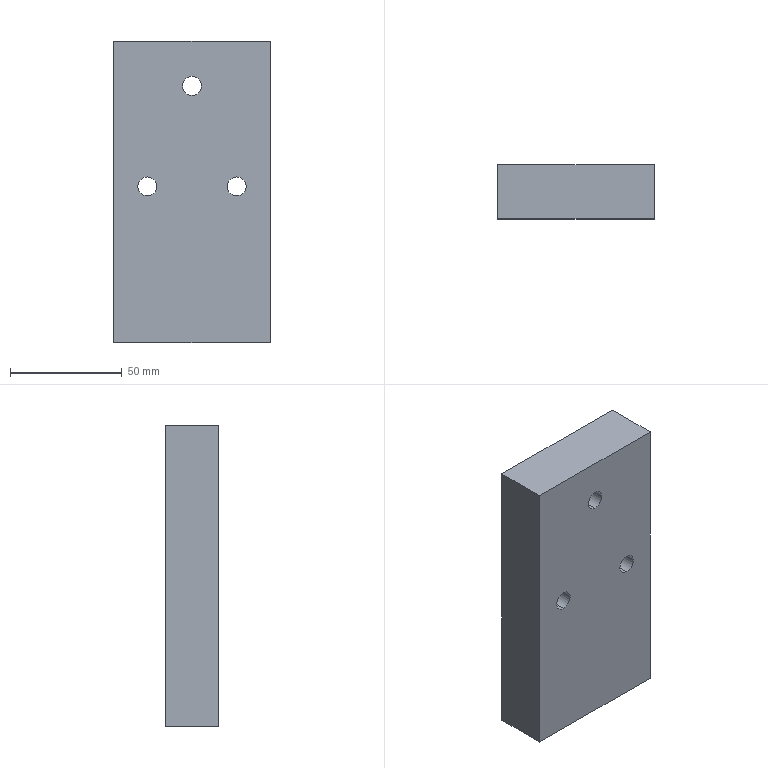Part | SolidWorks | features Extrusion 1, HoleWzd 1 | 1 solid | 12 faces | box 70 x 24 x 135 mm | volume 222714 mm3 | cylinder 6 | plane 6 | commonest cylinder face diameters 8.5 x6
STEP:
#1=CARTESIAN_POINT('',(-20.,0.,-1.75));
#2=VERTEX_POINT('',#1);
#3=CARTESIAN_POINT('',(-20.,0.,6.75));
#4=VERTEX_POINT('',#3);
#5=CARTESIAN_POINT('',(-20.,0.,2.5));
#6=DIRECTION('',(0.,1.,0.));
#7=DIRECTION('',(0.,0.,1.));
#8=AXIS2_PLACEMENT_3D('',#5,#6,#7);
#9=CIRCLE('',#8,4.25);
#10=EDGE_CURVE('',#2,#4,#9,.T.);
#11=ORIENTED_EDGE('',*,*,#10,.F.);
#12=CARTESIAN_POINT('',(-20.,24.,-1.75));
#13=VERTEX_POINT('',#12);
#14=CARTESIAN_POINT('',(-20.,24.,-1.75));
#15=DIRECTION('',(0.,1.,0.));
#16=VECTOR('',#15,1000.);
#17=LINE('',#14,#16);
#18=EDGE_CURVE('',#2,#13,#17,.T.);
#19=ORIENTED_EDGE('',*,*,#18,.T.);
#20=CARTESIAN_POINT('',(-20.,24.,6.75));
#21=VERTEX_POINT('',#20);
#22=CARTESIAN_POINT('',(-20.,24.,2.5));
#23=DIRECTION('',(0.,1.,0.));
#24=DIRECTION('',(0.,0.,1.));
#25=AXIS2_PLACEMENT_3D('',#22,#23,#24);
#26=CIRCLE('',#25,4.25);
#27=EDGE_CURVE('',#13,#21,#26,.T.);
#28=ORIENTED_EDGE('',*,*,#27,.T.);
#29=CARTESIAN_POINT('',(-20.,24.,6.75));
#30=DIRECTION('',(0.,1.,0.));
#31=VECTOR('',#30,1000.);
#32=LINE('',#29,#31);
#33=EDGE_CURVE('',#4,#21,#32,.T.);
#34=ORIENTED_EDGE('',*,*,#33,.F.);
#35=EDGE_LOOP('',(#11,#19,#28,#34));
#36=FACE_OUTER_BOUND('',#35,.T.);
#37=CARTESIAN_POINT('',(-20.,24.,2.5));
#38=DIRECTION('',(0.,1.,0.));
#39=DIRECTION('',(0.,0.,1.));
#40=AXIS2_PLACEMENT_3D('',#37,#38,#39);
#41=CYLINDRICAL_SURFACE('',#40,4.25);
#42=ADVANCED_FACE('',(#36),#41,.F.);
#43=CARTESIAN_POINT('',(20.,0.,-1.75));
#44=VERTEX_POINT('',#43);
#45=CARTESIAN_POINT('',(20.,0.,6.75));
#46=VERTEX_POINT('',#45);
#47=CARTESIAN_POINT('',(20.,0.,2.5));
#48=DIRECTION('',(0.,1.,0.));
#49=DIRECTION('',(0.,0.,1.));
#50=AXIS2_PLACEMENT_3D('',#47,#48,#49);
#51=CIRCLE('',#50,4.25);
#52=EDGE_CURVE('',#44,#46,#51,.T.);
#53=ORIENTED_EDGE('',*,*,#52,.F.);
#54=CARTESIAN_POINT('',(20.,24.,-1.75));
#55=VERTEX_POINT('',#54);
#56=CARTESIAN_POINT('',(20.,24.,-1.75));
#57=DIRECTION('',(0.,1.,0.));
#58=VECTOR('',#57,1000.);
#59=LINE('',#56,#58);
#60=EDGE_CURVE('',#44,#55,#59,.T.);
#61=ORIENTED_EDGE('',*,*,#60,.T.);
#62=CARTESIAN_POINT('',(20.,24.,6.75));
#63=VERTEX_POINT('',#62);
#64=CARTESIAN_POINT('',(20.,24.,2.5));
#65=DIRECTION('',(0.,1.,0.));
#66=DIRECTION('',(0.,0.,1.));
#67=AXIS2_PLACEMENT_3D('',#64,#65,#66);
#68=CIRCLE('',#67,4.25);
#69=EDGE_CURVE('',#55,#63,#68,.T.);
#70=ORIENTED_EDGE('',*,*,#69,.T.);
#71=CARTESIAN_POINT('',(20.,24.,6.75));
#72=DIRECTION('',(0.,1.,0.));
#73=VECTOR('',#72,1000.);
#74=LINE('',#71,#73);
#75=EDGE_CURVE('',#46,#63,#74,.T.);
#76=ORIENTED_EDGE('',*,*,#75,.F.);
#77=EDGE_LOOP('',(#53,#61,#70,#76));
#78=FACE_OUTER_BOUND('',#77,.T.);
#79=CARTESIAN_POINT('',(20.,24.,2.5));
#80=DIRECTION('',(0.,1.,0.));
#81=DIRECTION('',(0.,0.,1.));
#82=AXIS2_PLACEMENT_3D('',#79,#80,#81);
#83=CYLINDRICAL_SURFACE('',#82,4.25);
#84=ADVANCED_FACE('',(#78),#83,.F.);
#85=CARTESIAN_POINT('',(0.,0.,43.25));
#86=VERTEX_POINT('',#85);
#87=CARTESIAN_POINT('',(0.,0.,51.75));
#88=VERTEX_POINT('',#87);
#89=CARTESIAN_POINT('',(0.,0.,47.5));
#90=DIRECTION('',(0.,1.,0.));
#91=DIRECTION('',(0.,0.,1.));
#92=AXIS2_PLACEMENT_3D('',#89,#90,#91);
#93=CIRCLE('',#92,4.25);
#94=EDGE_CURVE('',#86,#88,#93,.T.);
#95=ORIENTED_EDGE('',*,*,#94,.F.);
#96=CARTESIAN_POINT('',(0.,24.,43.25));
#97=VERTEX_POINT('',#96);
#98=CARTESIAN_POINT('',(0.,24.,43.25));
#99=DIRECTION('',(0.,1.,0.));
#100=VECTOR('',#99,1000.);
#101=LINE('',#98,#100);
#102=EDGE_CURVE('',#86,#97,#101,.T.);
#103=ORIENTED_EDGE('',*,*,#102,.T.);
#104=CARTESIAN_POINT('',(0.,24.,51.75));
#105=VERTEX_POINT('',#104);
#106=CARTESIAN_POINT('',(0.,24.,47.5));
#107=DIRECTION('',(0.,1.,0.));
#108=DIRECTION('',(0.,0.,1.));
#109=AXIS2_PLACEMENT_3D('',#106,#107,#108);
#110=CIRCLE('',#109,4.25);
#111=EDGE_CURVE('',#97,#105,#110,.T.);
#112=ORIENTED_EDGE('',*,*,#111,.T.);
#113=CARTESIAN_POINT('',(0.,24.,51.75));
#114=DIRECTION('',(0.,1.,0.));
#115=VECTOR('',#114,1000.);
#116=LINE('',#113,#115);
#117=EDGE_CURVE('',#88,#105,#116,.T.);
#118=ORIENTED_EDGE('',*,*,#117,.F.);
#119=EDGE_LOOP('',(#95,#103,#112,#118));
#120=FACE_OUTER_BOUND('',#119,.T.);
#121=CARTESIAN_POINT('',(0.,24.,47.5));
#122=DIRECTION('',(0.,1.,0.));
#123=DIRECTION('',(0.,0.,1.));
#124=AXIS2_PLACEMENT_3D('',#121,#122,#123);
#125=CYLINDRICAL_SURFACE('',#124,4.25);
#126=ADVANCED_FACE('',(#120),#125,.F.);
#127=CARTESIAN_POINT('',(35.,0.,67.5));
#128=VERTEX_POINT('',#127);
#129=CARTESIAN_POINT('',(35.,0.,-67.5));
#130=VERTEX_POINT('',#129);
#131=CARTESIAN_POINT('',(35.,0.,67.5));
#132=DIRECTION('',(0.,0.,-1.));
#133=VECTOR('',#132,1000.);
#134=LINE('',#131,#133);
#135=EDGE_CURVE('',#128,#130,#134,.T.);
#136=ORIENTED_EDGE('',*,*,#135,.T.);
#137=CARTESIAN_POINT('',(35.,24.,-67.5));
#138=VERTEX_POINT('',#137);
#139=CARTESIAN_POINT('',(35.,24.,-67.5));
#140=DIRECTION('',(0.,-1.,0.));
#141=VECTOR('',#140,1000.);
#142=LINE('',#139,#141);
#143=EDGE_CURVE('',#138,#130,#142,.T.);
#144=ORIENTED_EDGE('',*,*,#143,.F.);
#145=CARTESIAN_POINT('',(35.,24.,67.5));
#146=VERTEX_POINT('',#145);
#147=CARTESIAN_POINT('',(35.,24.,67.5));
#148=DIRECTION('',(0.,0.,-1.));
#149=VECTOR('',#148,1000.);
#150=LINE('',#147,#149);
#151=EDGE_CURVE('',#146,#138,#150,.T.);
#152=ORIENTED_EDGE('',*,*,#151,.F.);
#153=CARTESIAN_POINT('',(35.,24.,67.5));
#154=DIRECTION('',(0.,-1.,0.));
#155=VECTOR('',#154,1000.);
#156=LINE('',#153,#155);
#157=EDGE_CURVE('',#146,#128,#156,.T.);
#158=ORIENTED_EDGE('',*,*,#157,.T.);
#159=EDGE_LOOP('',(#136,#144,#152,#158));
#160=FACE_OUTER_BOUND('',#159,.T.);
#161=CARTESIAN_POINT('',(35.,24.,67.5));
#162=DIRECTION('',(-1.,0.,0.));
#163=DIRECTION('',(0.,0.,1.));
#164=AXIS2_PLACEMENT_3D('',#161,#162,#163);
#165=PLANE('',#164);
#166=ADVANCED_FACE('',(#160),#165,.F.);
#167=CARTESIAN_POINT('',(-35.,0.,-67.5));
#168=VERTEX_POINT('',#167);
#169=CARTESIAN_POINT('',(-35.,0.,-67.5));
#170=DIRECTION('',(-1.,0.,0.));
#171=VECTOR('',#170,1000.);
#172=LINE('',#169,#171);
#173=EDGE_CURVE('',#130,#168,#172,.T.);
#174=ORIENTED_EDGE('',*,*,#173,.T.);
#175=CARTESIAN_POINT('',(-35.,24.,-67.5));
#176=VERTEX_POINT('',#175);
#177=CARTESIAN_POINT('',(-35.,24.,-67.5));
#178=DIRECTION('',(0.,-1.,0.));
#179=VECTOR('',#178,1000.);
#180=LINE('',#177,#179);
#181=EDGE_CURVE('',#176,#168,#180,.T.);
#182=ORIENTED_EDGE('',*,*,#181,.F.);
#183=CARTESIAN_POINT('',(-35.,24.,-67.5));
#184=DIRECTION('',(-1.,0.,0.));
#185=VECTOR('',#184,1000.);
#186=LINE('',#183,#185);
#187=EDGE_CURVE('',#138,#176,#186,.T.);
#188=ORIENTED_EDGE('',*,*,#187,.F.);
#189=ORIENTED_EDGE('',*,*,#143,.T.);
#190=EDGE_LOOP('',(#174,#182,#188,#189));
#191=FACE_OUTER_BOUND('',#190,.T.);
#192=CARTESIAN_POINT('',(-35.,24.,-67.5));
#193=DIRECTION('',(0.,0.,1.));
#194=DIRECTION('',(1.,0.,0.));
#195=AXIS2_PLACEMENT_3D('',#192,#193,#194);
#196=PLANE('',#195);
#197=ADVANCED_FACE('',(#191),#196,.F.);
#198=CARTESIAN_POINT('',(-35.,0.,67.5));
#199=VERTEX_POINT('',#198);
#200=CARTESIAN_POINT('',(-35.,0.,67.5));
#201=DIRECTION('',(0.,0.,1.));
#202=VECTOR('',#201,1000.);
#203=LINE('',#200,#202);
#204=EDGE_CURVE('',#168,#199,#203,.T.);
#205=ORIENTED_EDGE('',*,*,#204,.T.);
#206=CARTESIAN_POINT('',(-35.,24.,67.5));
#207=VERTEX_POINT('',#206);
#208=CARTESIAN_POINT('',(-35.,24.,67.5));
#209=DIRECTION('',(0.,-1.,0.));
#210=VECTOR('',#209,1000.);
#211=LINE('',#208,#210);
#212=EDGE_CURVE('',#207,#199,#211,.T.);
#213=ORIENTED_EDGE('',*,*,#212,.F.);
#214=CARTESIAN_POINT('',(-35.,24.,67.5));
#215=DIRECTION('',(0.,0.,1.));
#216=VECTOR('',#215,1000.);
#217=LINE('',#214,#216);
#218=EDGE_CURVE('',#176,#207,#217,.T.);
#219=ORIENTED_EDGE('',*,*,#218,.F.);
#220=ORIENTED_EDGE('',*,*,#181,.T.);
#221=EDGE_LOOP('',(#205,#213,#219,#220));
#222=FACE_OUTER_BOUND('',#221,.T.);
#223=CARTESIAN_POINT('',(-35.,24.,67.5));
#224=DIRECTION('',(1.,0.,0.));
#225=DIRECTION('',(0.,0.,-1.));
#226=AXIS2_PLACEMENT_3D('',#223,#224,#225);
#227=PLANE('',#226);
#228=ADVANCED_FACE('',(#222),#227,.F.);
#229=CARTESIAN_POINT('',(-35.,0.,67.5));
#230=DIRECTION('',(1.,0.,0.));
#231=VECTOR('',#230,1000.);
#232=LINE('',#229,#231);
#233=EDGE_CURVE('',#199,#128,#232,.T.);
#234=ORIENTED_EDGE('',*,*,#233,.T.);
#235=ORIENTED_EDGE('',*,*,#157,.F.);
#236=CARTESIAN_POINT('',(-35.,24.,67.5));
#237=DIRECTION('',(1.,0.,0.));
#238=VECTOR('',#237,1000.);
#239=LINE('',#236,#238);
#240=EDGE_CURVE('',#207,#146,#239,.T.);
#241=ORIENTED_EDGE('',*,*,#240,.F.);
#242=ORIENTED_EDGE('',*,*,#212,.T.);
#243=EDGE_LOOP('',(#234,#235,#241,#242));
#244=FACE_OUTER_BOUND('',#243,.T.);
#245=CARTESIAN_POINT('',(-35.,24.,67.5));
#246=DIRECTION('',(0.,0.,-1.));
#247=DIRECTION('',(-1.,0.,0.));
#248=AXIS2_PLACEMENT_3D('',#245,#246,#247);
#249=PLANE('',#248);
#250=ADVANCED_FACE('',(#244),#249,.F.);
#251=CARTESIAN_POINT('',(-20.,24.,2.5));
#252=DIRECTION('',(0.,1.,0.));
#253=DIRECTION('',(0.,0.,1.));
#254=AXIS2_PLACEMENT_3D('',#251,#252,#253);
#255=CIRCLE('',#254,4.25);
#256=EDGE_CURVE('',#21,#13,#255,.T.);
#257=ORIENTED_EDGE('',*,*,#256,.F.);
#258=ORIENTED_EDGE('',*,*,#27,.F.);
#259=EDGE_LOOP('',(#257,#258));
#260=FACE_BOUND('',#259,.T.);
#261=CARTESIAN_POINT('',(20.,24.,2.5));
#262=DIRECTION('',(0.,1.,0.));
#263=DIRECTION('',(0.,0.,1.));
#264=AXIS2_PLACEMENT_3D('',#261,#262,#263);
#265=CIRCLE('',#264,4.25);
#266=EDGE_CURVE('',#63,#55,#265,.T.);
#267=ORIENTED_EDGE('',*,*,#266,.F.);
#268=ORIENTED_EDGE('',*,*,#69,.F.);
#269=EDGE_LOOP('',(#267,#268));
#270=FACE_BOUND('',#269,.T.);
#271=CARTESIAN_POINT('',(0.,24.,47.5));
#272=DIRECTION('',(0.,1.,0.));
#273=DIRECTION('',(0.,0.,1.));
#274=AXIS2_PLACEMENT_3D('',#271,#272,#273);
#275=CIRCLE('',#274,4.25);
#276=EDGE_CURVE('',#105,#97,#275,.T.);
#277=ORIENTED_EDGE('',*,*,#276,.F.);
#278=ORIENTED_EDGE('',*,*,#111,.F.);
#279=EDGE_LOOP('',(#277,#278));
#280=FACE_BOUND('',#279,.T.);
#281=ORIENTED_EDGE('',*,*,#151,.T.);
#282=ORIENTED_EDGE('',*,*,#187,.T.);
#283=ORIENTED_EDGE('',*,*,#218,.T.);
#284=ORIENTED_EDGE('',*,*,#240,.T.);
#285=EDGE_LOOP('',(#281,#282,#283,#284));
#286=FACE_OUTER_BOUND('',#285,.T.);
#287=CARTESIAN_POINT('',(0.,24.,0.));
#288=DIRECTION('',(0.,-1.,0.));
#289=DIRECTION('',(0.,0.,-1.));
#290=AXIS2_PLACEMENT_3D('',#287,#288,#289);
#291=PLANE('',#290);
#292=ADVANCED_FACE('',(#260,#270,#280,#286),#291,.F.);
#293=CARTESIAN_POINT('',(-20.,0.,2.5));
#294=DIRECTION('',(0.,1.,0.));
#295=DIRECTION('',(0.,0.,1.));
#296=AXIS2_PLACEMENT_3D('',#293,#294,#295);
#297=CIRCLE('',#296,4.25);
#298=EDGE_CURVE('',#4,#2,#297,.T.);
#299=ORIENTED_EDGE('',*,*,#298,.T.);
#300=ORIENTED_EDGE('',*,*,#10,.T.);
#301=EDGE_LOOP('',(#299,#300));
#302=FACE_BOUND('',#301,.T.);
#303=CARTESIAN_POINT('',(20.,0.,2.5));
#304=DIRECTION('',(0.,1.,0.));
#305=DIRECTION('',(0.,0.,1.));
#306=AXIS2_PLACEMENT_3D('',#303,#304,#305);
#307=CIRCLE('',#306,4.25);
#308=EDGE_CURVE('',#46,#44,#307,.T.);
#309=ORIENTED_EDGE('',*,*,#308,.T.);
#310=ORIENTED_EDGE('',*,*,#52,.T.);
#311=EDGE_LOOP('',(#309,#310));
#312=FACE_BOUND('',#311,.T.);
#313=CARTESIAN_POINT('',(0.,0.,47.5));
#314=DIRECTION('',(0.,1.,0.));
#315=DIRECTION('',(0.,0.,1.));
#316=AXIS2_PLACEMENT_3D('',#313,#314,#315);
#317=CIRCLE('',#316,4.25);
#318=EDGE_CURVE('',#88,#86,#317,.T.);
#319=ORIENTED_EDGE('',*,*,#318,.T.);
#320=ORIENTED_EDGE('',*,*,#94,.T.);
#321=EDGE_LOOP('',(#319,#320));
#322=FACE_BOUND('',#321,.T.);
#323=ORIENTED_EDGE('',*,*,#135,.F.);
#324=ORIENTED_EDGE('',*,*,#233,.F.);
#325=ORIENTED_EDGE('',*,*,#204,.F.);
#326=ORIENTED_EDGE('',*,*,#173,.F.);
#327=EDGE_LOOP('',(#323,#324,#325,#326));
#328=FACE_OUTER_BOUND('',#327,.T.);
#329=CARTESIAN_POINT('',(0.,0.,0.));
#330=DIRECTION('',(0.,-1.,0.));
#331=DIRECTION('',(0.,0.,-1.));
#332=AXIS2_PLACEMENT_3D('',#329,#330,#331);
#333=PLANE('',#332);
#334=ADVANCED_FACE('',(#302,#312,#322,#328),#333,.T.);
#335=ORIENTED_EDGE('',*,*,#102,.F.);
#336=ORIENTED_EDGE('',*,*,#318,.F.);
#337=ORIENTED_EDGE('',*,*,#117,.T.);
#338=ORIENTED_EDGE('',*,*,#276,.T.);
#339=EDGE_LOOP('',(#335,#336,#337,#338));
#340=FACE_OUTER_BOUND('',#339,.T.);
#341=CARTESIAN_POINT('',(0.,24.,47.5));
#342=DIRECTION('',(0.,1.,0.));
#343=DIRECTION('',(0.,0.,1.));
#344=AXIS2_PLACEMENT_3D('',#341,#342,#343);
#345=CYLINDRICAL_SURFACE('',#344,4.25);
#346=ADVANCED_FACE('',(#340),#345,.F.);
#347=ORIENTED_EDGE('',*,*,#60,.F.);
#348=ORIENTED_EDGE('',*,*,#308,.F.);
#349=ORIENTED_EDGE('',*,*,#75,.T.);
#350=ORIENTED_EDGE('',*,*,#266,.T.);
#351=EDGE_LOOP('',(#347,#348,#349,#350));
#352=FACE_OUTER_BOUND('',#351,.T.);
#353=CARTESIAN_POINT('',(20.,24.,2.5));
#354=DIRECTION('',(0.,1.,0.));
#355=DIRECTION('',(0.,0.,1.));
#356=AXIS2_PLACEMENT_3D('',#353,#354,#355);
#357=CYLINDRICAL_SURFACE('',#356,4.25);
#358=ADVANCED_FACE('',(#352),#357,.F.);
#359=ORIENTED_EDGE('',*,*,#18,.F.);
#360=ORIENTED_EDGE('',*,*,#298,.F.);
#361=ORIENTED_EDGE('',*,*,#33,.T.);
#362=ORIENTED_EDGE('',*,*,#256,.T.);
#363=EDGE_LOOP('',(#359,#360,#361,#362));
#364=FACE_OUTER_BOUND('',#363,.T.);
#365=CARTESIAN_POINT('',(-20.,24.,2.5));
#366=DIRECTION('',(0.,1.,0.));
#367=DIRECTION('',(0.,0.,1.));
#368=AXIS2_PLACEMENT_3D('',#365,#366,#367);
#369=CYLINDRICAL_SURFACE('',#368,4.25);
#370=ADVANCED_FACE('',(#364),#369,.F.);
#371=CLOSED_SHELL('',(#42,#84,#126,#166,#197,#228,#250,#292,#334,#346,#358,#370));
#372=MANIFOLD_SOLID_BREP('',#371);
#373=CARTESIAN_POINT('',(0.,0.,0.));
#374=DIRECTION('',(0.,0.,1.));
#375=DIRECTION('',(1.,0.,0.));
#376=AXIS2_PLACEMENT_3D('',#373,#374,#375);
#377=(LENGTH_UNIT()NAMED_UNIT(*)SI_UNIT(.MILLI.,.METRE.));
#378=UNCERTAINTY_MEASURE_WITH_UNIT(LENGTH_MEASURE(0.00001),#377,'','');
#379=(NAMED_UNIT(*)PLANE_ANGLE_UNIT()SI_UNIT($,.RADIAN.));
#380=(NAMED_UNIT(*)SI_UNIT($,.STERADIAN.)SOLID_ANGLE_UNIT());
#381=(GEOMETRIC_REPRESENTATION_CONTEXT(3)GLOBAL_UNCERTAINTY_ASSIGNED_CONTEXT((#378))GLOBAL_UNIT_ASSIGNED_CONTEXT((#377,#379,#380))REPRESENTATION_CONTEXT('',''));
#382=ADVANCED_BREP_SHAPE_REPRESENTATION('',(#372,#376),#381);